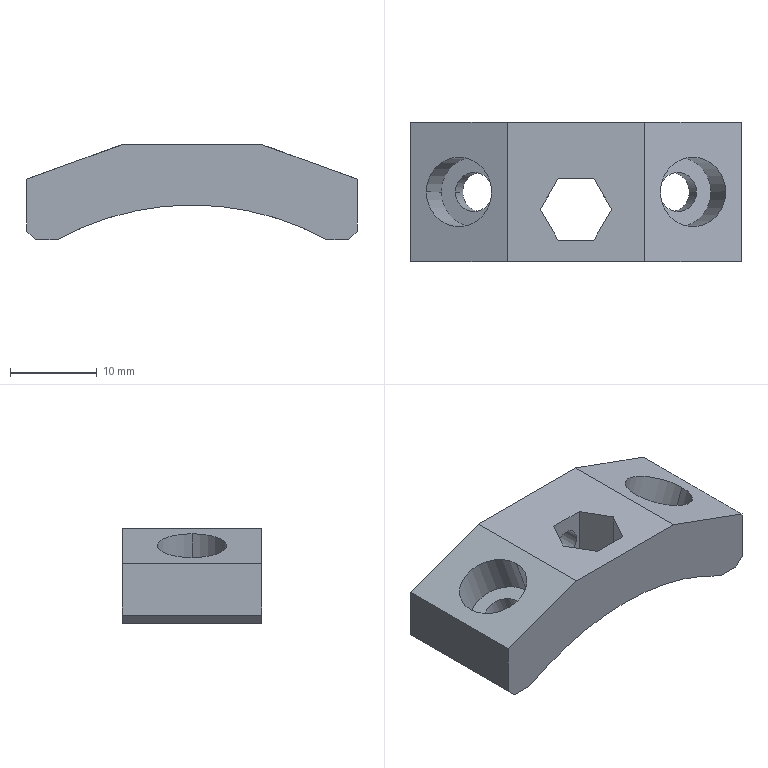Part | SolidWorks | features HoleWzd 2, Chamfer 1, Extrusion 1, ICE 1, MirrorPattern 1 | 1 solid | 30 faces | box 38 x 16 x 11 mm | volume 3676 mm3 | plane 19 | cylinder 11 | commonest cylinder face diameters 4.5 x4 8 x4 3.3 x2 64 x1
STEP:
#1=CARTESIAN_POINT('',(7.992,0.,33.654));
#2=VERTEX_POINT('',#1);
#3=CARTESIAN_POINT('',(15.51,0.,30.917));
#4=VERTEX_POINT('',#3);
#5=CARTESIAN_POINT('',(11.751,0.,32.286));
#6=DIRECTION('',(0.342,0.,0.9397));
#7=DIRECTION('',(0.9397,0.,-0.342));
#8=AXIS2_PLACEMENT_3D('',#5,#6,#7);
#9=CIRCLE('',#8,4.);
#10=EDGE_CURVE('',#2,#4,#9,.T.);
#11=ORIENTED_EDGE('',*,*,#10,.F.);
#12=CARTESIAN_POINT('',(9.702,0.,38.352));
#13=VERTEX_POINT('',#12);
#14=CARTESIAN_POINT('',(9.702,0.,38.352));
#15=DIRECTION('',(0.342,0.,0.9397));
#16=VECTOR('',#15,1000.);
#17=LINE('',#14,#16);
#18=EDGE_CURVE('',#2,#13,#17,.T.);
#19=ORIENTED_EDGE('',*,*,#18,.T.);
#20=CARTESIAN_POINT('',(17.22,0.,35.616));
#21=VERTEX_POINT('',#20);
#22=CARTESIAN_POINT('',(13.461,0.,36.984));
#23=DIRECTION('',(0.342,0.,0.9397));
#24=DIRECTION('',(0.9397,0.,-0.342));
#25=AXIS2_PLACEMENT_3D('',#22,#23,#24);
#26=CIRCLE('',#25,4.);
#27=EDGE_CURVE('',#13,#21,#26,.T.);
#28=ORIENTED_EDGE('',*,*,#27,.T.);
#29=CARTESIAN_POINT('',(17.22,0.,35.616));
#30=DIRECTION('',(0.342,0.,0.9397));
#31=VECTOR('',#30,1000.);
#32=LINE('',#29,#31);
#33=EDGE_CURVE('',#4,#21,#32,.T.);
#34=ORIENTED_EDGE('',*,*,#33,.F.);
#35=EDGE_LOOP('',(#11,#19,#28,#34));
#36=FACE_OUTER_BOUND('',#35,.T.);
#37=CARTESIAN_POINT('',(13.461,0.,36.984));
#38=DIRECTION('',(0.342,0.,0.9397));
#39=DIRECTION('',(0.9397,0.,-0.342));
#40=AXIS2_PLACEMENT_3D('',#37,#38,#39);
#41=CYLINDRICAL_SURFACE('',#40,4.);
#42=ADVANCED_FACE('',(#36),#41,.F.);
#43=CARTESIAN_POINT('',(8.803,0.,30.765));
#44=VERTEX_POINT('',#43);
#45=CARTESIAN_POINT('',(13.032,0.,29.226));
#46=VERTEX_POINT('',#45);
#47=CARTESIAN_POINT('',(8.803,0.,30.765));
#48=CARTESIAN_POINT('',(8.803,-0.1468,30.765));
#49=CARTESIAN_POINT('',(8.817,-0.2928,30.761));
#50=CARTESIAN_POINT('',(8.872,-0.583,30.745));
#51=CARTESIAN_POINT('',(8.914,-0.7251,30.733));
#52=CARTESIAN_POINT('',(9.076,-1.131,30.686));
#53=CARTESIAN_POINT('',(9.237,-1.382,30.639));
#54=CARTESIAN_POINT('',(9.534,-1.694,30.547));
#55=CARTESIAN_POINT('',(9.645,-1.789,30.512));
#56=CARTESIAN_POINT('',(9.878,-1.952,30.438));
#57=CARTESIAN_POINT('',(10.001,-2.021,30.398));
#58=CARTESIAN_POINT('',(10.259,-2.134,30.311));
#59=CARTESIAN_POINT('',(10.394,-2.178,30.265));
#60=CARTESIAN_POINT('',(10.666,-2.235,30.171));
#61=CARTESIAN_POINT('',(10.803,-2.25,30.122));
#62=CARTESIAN_POINT('',(11.082,-2.25,30.02));
#63=CARTESIAN_POINT('',(11.22,-2.236,29.969));
#64=CARTESIAN_POINT('',(11.489,-2.179,29.867));
#65=CARTESIAN_POINT('',(11.622,-2.136,29.815));
#66=CARTESIAN_POINT('',(11.876,-2.023,29.715));
#67=CARTESIAN_POINT('',(11.996,-1.954,29.667));
#68=CARTESIAN_POINT('',(12.222,-1.791,29.574));
#69=CARTESIAN_POINT('',(12.329,-1.696,29.53));
#70=CARTESIAN_POINT('',(12.521,-1.488,29.449));
#71=CARTESIAN_POINT('',(12.607,-1.375,29.412));
#72=CARTESIAN_POINT('',(12.758,-1.13,29.347));
#73=CARTESIAN_POINT('',(12.822,-0.9987,29.319));
#74=CARTESIAN_POINT('',(12.977,-0.5928,29.251));
#75=CARTESIAN_POINT('',(13.032,-0.2974,29.226));
#76=CARTESIAN_POINT('',(13.032,0.,29.226));
#77=B_SPLINE_CURVE_WITH_KNOTS('',3,(#47,#48,#49,#50,#51,#52,#53,#54,#55,#56,#57,#58,#59,#60,#61,#62,#63,#64,#65,#66,#67,#68,#69,#70,#71,#72,#73,#74,#75,#76),.UNSPECIFIED.,.F.,.F.,(4,2,2,2,2,2,2,2,2,2,2,2,2,2,4),(0.007037,0.007476,0.007916,0.008795,0.009235,0.009675,0.01011,0.01055,0.01099,0.01143,0.01187,0.01231,0.01275,0.01319,0.01407),.UNSPECIFIED.);
#78=EDGE_CURVE('',#44,#46,#77,.T.);
#79=ORIENTED_EDGE('',*,*,#78,.F.);
#80=CARTESIAN_POINT('',(9.637,0.,33.055));
#81=VERTEX_POINT('',#80);
#82=CARTESIAN_POINT('',(11.347,0.,37.754));
#83=DIRECTION('',(0.342,0.,0.9397));
#84=VECTOR('',#83,1000.);
#85=LINE('',#82,#84);
#86=EDGE_CURVE('',#44,#81,#85,.T.);
#87=ORIENTED_EDGE('',*,*,#86,.T.);
#88=CARTESIAN_POINT('',(13.865,0.,31.516));
#89=VERTEX_POINT('',#88);
#90=CARTESIAN_POINT('',(11.751,0.,32.286));
#91=DIRECTION('',(0.342,0.,0.9397));
#92=DIRECTION('',(0.9397,0.,-0.342));
#93=AXIS2_PLACEMENT_3D('',#90,#91,#92);
#94=CIRCLE('',#93,2.25);
#95=EDGE_CURVE('',#81,#89,#94,.T.);
#96=ORIENTED_EDGE('',*,*,#95,.T.);
#97=CARTESIAN_POINT('',(15.575,0.,36.214));
#98=DIRECTION('',(0.342,0.,0.9397));
#99=VECTOR('',#98,1000.);
#100=LINE('',#97,#99);
#101=EDGE_CURVE('',#46,#89,#100,.T.);
#102=ORIENTED_EDGE('',*,*,#101,.F.);
#103=EDGE_LOOP('',(#79,#87,#96,#102));
#104=FACE_OUTER_BOUND('',#103,.T.);
#105=CARTESIAN_POINT('',(13.461,0.,36.984));
#106=DIRECTION('',(0.342,0.,0.9397));
#107=DIRECTION('',(0.9397,0.,-0.342));
#108=AXIS2_PLACEMENT_3D('',#105,#106,#107);
#109=CYLINDRICAL_SURFACE('',#108,2.25);
#110=ADVANCED_FACE('',(#104),#109,.F.);
#111=CARTESIAN_POINT('',(-15.51,0.,30.917));
#112=VERTEX_POINT('',#111);
#113=CARTESIAN_POINT('',(-7.992,0.,33.654));
#114=VERTEX_POINT('',#113);
#115=CARTESIAN_POINT('',(-11.751,0.,32.286));
#116=DIRECTION('',(-0.342,0.,0.9397));
#117=DIRECTION('',(0.9397,0.,0.342));
#118=AXIS2_PLACEMENT_3D('',#115,#116,#117);
#119=CIRCLE('',#118,4.);
#120=EDGE_CURVE('',#112,#114,#119,.T.);
#121=ORIENTED_EDGE('',*,*,#120,.F.);
#122=CARTESIAN_POINT('',(-17.22,0.,35.616));
#123=VERTEX_POINT('',#122);
#124=CARTESIAN_POINT('',(-17.22,0.,35.616));
#125=DIRECTION('',(-0.342,0.,0.9397));
#126=VECTOR('',#125,1000.);
#127=LINE('',#124,#126);
#128=EDGE_CURVE('',#112,#123,#127,.T.);
#129=ORIENTED_EDGE('',*,*,#128,.T.);
#130=CARTESIAN_POINT('',(-9.702,0.,38.352));
#131=VERTEX_POINT('',#130);
#132=CARTESIAN_POINT('',(-13.461,0.,36.984));
#133=DIRECTION('',(-0.342,0.,0.9397));
#134=DIRECTION('',(0.9397,0.,0.342));
#135=AXIS2_PLACEMENT_3D('',#132,#133,#134);
#136=CIRCLE('',#135,4.);
#137=EDGE_CURVE('',#123,#131,#136,.T.);
#138=ORIENTED_EDGE('',*,*,#137,.T.);
#139=CARTESIAN_POINT('',(-9.702,0.,38.352));
#140=DIRECTION('',(-0.342,0.,0.9397));
#141=VECTOR('',#140,1000.);
#142=LINE('',#139,#141);
#143=EDGE_CURVE('',#114,#131,#142,.T.);
#144=ORIENTED_EDGE('',*,*,#143,.F.);
#145=EDGE_LOOP('',(#121,#129,#138,#144));
#146=FACE_OUTER_BOUND('',#145,.T.);
#147=CARTESIAN_POINT('',(-13.461,0.,36.984));
#148=DIRECTION('',(-0.342,0.,0.9397));
#149=DIRECTION('',(0.9397,0.,0.342));
#150=AXIS2_PLACEMENT_3D('',#147,#148,#149);
#151=CYLINDRICAL_SURFACE('',#150,4.);
#152=ADVANCED_FACE('',(#146),#151,.F.);
#153=CARTESIAN_POINT('',(-13.032,0.,29.226));
#154=VERTEX_POINT('',#153);
#155=CARTESIAN_POINT('',(-8.803,0.,30.765));
#156=VERTEX_POINT('',#155);
#157=CARTESIAN_POINT('',(-13.032,0.,29.226));
#158=CARTESIAN_POINT('',(-13.032,-0.1468,29.226));
#159=CARTESIAN_POINT('',(-13.019,-0.2928,29.232));
#160=CARTESIAN_POINT('',(-12.966,-0.583,29.255));
#161=CARTESIAN_POINT('',(-12.927,-0.7251,29.273));
#162=CARTESIAN_POINT('',(-12.772,-1.131,29.341));
#163=CARTESIAN_POINT('',(-12.618,-1.382,29.408));
#164=CARTESIAN_POINT('',(-12.332,-1.694,29.529));
#165=CARTESIAN_POINT('',(-12.225,-1.789,29.573));
#166=CARTESIAN_POINT('',(-11.998,-1.952,29.666));
#167=CARTESIAN_POINT('',(-11.878,-2.021,29.714));
#168=CARTESIAN_POINT('',(-11.625,-2.134,29.814));
#169=CARTESIAN_POINT('',(-11.492,-2.178,29.866));
#170=CARTESIAN_POINT('',(-11.223,-2.235,29.968));
#171=CARTESIAN_POINT('',(-11.086,-2.25,30.019));
#172=CARTESIAN_POINT('',(-10.807,-2.25,30.12));
#173=CARTESIAN_POINT('',(-10.669,-2.236,30.17));
#174=CARTESIAN_POINT('',(-10.397,-2.179,30.264));
#175=CARTESIAN_POINT('',(-10.262,-2.136,30.31));
#176=CARTESIAN_POINT('',(-10.003,-2.023,30.397));
#177=CARTESIAN_POINT('',(-9.88,-1.954,30.437));
#178=CARTESIAN_POINT('',(-9.647,-1.791,30.511));
#179=CARTESIAN_POINT('',(-9.537,-1.696,30.546));
#180=CARTESIAN_POINT('',(-9.338,-1.488,30.607));
#181=CARTESIAN_POINT('',(-9.248,-1.375,30.634));
#182=CARTESIAN_POINT('',(-9.091,-1.13,30.682));
#183=CARTESIAN_POINT('',(-9.023,-0.9987,30.702));
#184=CARTESIAN_POINT('',(-8.861,-0.5928,30.749));
#185=CARTESIAN_POINT('',(-8.803,-0.2974,30.765));
#186=CARTESIAN_POINT('',(-8.803,0.,30.765));
#187=B_SPLINE_CURVE_WITH_KNOTS('',3,(#157,#158,#159,#160,#161,#162,#163,#164,#165,#166,#167,#168,#169,#170,#171,#172,#173,#174,#175,#176,#177,#178,#179,#180,#181,#182,#183,#184,#185,#186),.UNSPECIFIED.,.F.,.F.,(4,2,2,2,2,2,2,2,2,2,2,2,2,2,4),(0.007037,0.007476,0.007916,0.008795,0.009235,0.009675,0.01011,0.01055,0.01099,0.01143,0.01187,0.01231,0.01275,0.01319,0.01407),.UNSPECIFIED.);
#188=EDGE_CURVE('',#154,#156,#187,.T.);
#189=ORIENTED_EDGE('',*,*,#188,.F.);
#190=CARTESIAN_POINT('',(-13.865,0.,31.516));
#191=VERTEX_POINT('',#190);
#192=CARTESIAN_POINT('',(-15.575,0.,36.214));
#193=DIRECTION('',(-0.342,0.,0.9397));
#194=VECTOR('',#193,1000.);
#195=LINE('',#192,#194);
#196=EDGE_CURVE('',#154,#191,#195,.T.);
#197=ORIENTED_EDGE('',*,*,#196,.T.);
#198=CARTESIAN_POINT('',(-9.637,0.,33.055));
#199=VERTEX_POINT('',#198);
#200=CARTESIAN_POINT('',(-11.751,0.,32.286));
#201=DIRECTION('',(-0.342,0.,0.9397));
#202=DIRECTION('',(0.9397,0.,0.342));
#203=AXIS2_PLACEMENT_3D('',#200,#201,#202);
#204=CIRCLE('',#203,2.25);
#205=EDGE_CURVE('',#191,#199,#204,.T.);
#206=ORIENTED_EDGE('',*,*,#205,.T.);
#207=CARTESIAN_POINT('',(-11.347,0.,37.754));
#208=DIRECTION('',(-0.342,0.,0.9397));
#209=VECTOR('',#208,1000.);
#210=LINE('',#207,#209);
#211=EDGE_CURVE('',#156,#199,#210,.T.);
#212=ORIENTED_EDGE('',*,*,#211,.F.);
#213=EDGE_LOOP('',(#189,#197,#206,#212));
#214=FACE_OUTER_BOUND('',#213,.T.);
#215=CARTESIAN_POINT('',(-13.461,0.,36.984));
#216=DIRECTION('',(-0.342,0.,0.9397));
#217=DIRECTION('',(0.9397,0.,0.342));
#218=AXIS2_PLACEMENT_3D('',#215,#216,#217);
#219=CYLINDRICAL_SURFACE('',#218,2.25);
#220=ADVANCED_FACE('',(#214),#219,.F.);
#221=CARTESIAN_POINT('',(0.,1.55,33.85));
#222=VERTEX_POINT('',#221);
#223=CARTESIAN_POINT('',(0.,1.55,37.15));
#224=VERTEX_POINT('',#223);
#225=CARTESIAN_POINT('',(0.,1.55,35.5));
#226=DIRECTION('',(0.,1.,0.));
#227=DIRECTION('',(-1.,0.,0.));
#228=AXIS2_PLACEMENT_3D('',#225,#226,#227);
#229=CIRCLE('',#228,1.65);
#230=EDGE_CURVE('',#222,#224,#229,.T.);
#231=ORIENTED_EDGE('',*,*,#230,.F.);
#232=CARTESIAN_POINT('',(0.,8.,33.85));
#233=VERTEX_POINT('',#232);
#234=CARTESIAN_POINT('',(0.,8.,33.85));
#235=DIRECTION('',(0.,1.,0.));
#236=VECTOR('',#235,1000.);
#237=LINE('',#234,#236);
#238=EDGE_CURVE('',#222,#233,#237,.T.);
#239=ORIENTED_EDGE('',*,*,#238,.T.);
#240=CARTESIAN_POINT('',(0.,8.,37.15));
#241=VERTEX_POINT('',#240);
#242=CARTESIAN_POINT('',(0.,8.,35.5));
#243=DIRECTION('',(0.,1.,0.));
#244=DIRECTION('',(0.,0.,1.));
#245=AXIS2_PLACEMENT_3D('',#242,#243,#244);
#246=CIRCLE('',#245,1.65);
#247=EDGE_CURVE('',#233,#241,#246,.T.);
#248=ORIENTED_EDGE('',*,*,#247,.T.);
#249=CARTESIAN_POINT('',(0.,8.,37.15));
#250=DIRECTION('',(0.,1.,0.));
#251=VECTOR('',#250,1000.);
#252=LINE('',#249,#251);
#253=EDGE_CURVE('',#224,#241,#252,.T.);
#254=ORIENTED_EDGE('',*,*,#253,.F.);
#255=EDGE_LOOP('',(#231,#239,#248,#254));
#256=FACE_OUTER_BOUND('',#255,.T.);
#257=CARTESIAN_POINT('',(0.,8.,35.5));
#258=DIRECTION('',(0.,1.,0.));
#259=DIRECTION('',(0.,0.,1.));
#260=AXIS2_PLACEMENT_3D('',#257,#258,#259);
#261=CYLINDRICAL_SURFACE('',#260,1.65);
#262=ADVANCED_FACE('',(#256),#261,.F.);
#263=CARTESIAN_POINT('',(-13.461,0.,36.984));
#264=DIRECTION('',(-0.342,0.,0.9397));
#265=DIRECTION('',(0.9397,0.,0.342));
#266=AXIS2_PLACEMENT_3D('',#263,#264,#265);
#267=CIRCLE('',#266,4.);
#268=EDGE_CURVE('',#131,#123,#267,.T.);
#269=ORIENTED_EDGE('',*,*,#268,.F.);
#270=ORIENTED_EDGE('',*,*,#137,.F.);
#271=EDGE_LOOP('',(#269,#270));
#272=FACE_BOUND('',#271,.T.);
#273=CARTESIAN_POINT('',(-19.,-8.,34.968));
#274=VERTEX_POINT('',#273);
#275=CARTESIAN_POINT('',(-7.922,-8.,39.));
#276=VERTEX_POINT('',#275);
#277=CARTESIAN_POINT('',(-7.922,-8.,39.));
#278=DIRECTION('',(0.9397,0.,0.342));
#279=VECTOR('',#278,1000.);
#280=LINE('',#277,#279);
#281=EDGE_CURVE('',#274,#276,#280,.T.);
#282=ORIENTED_EDGE('',*,*,#281,.T.);
#283=CARTESIAN_POINT('',(-7.922,8.,39.));
#284=VERTEX_POINT('',#283);
#285=CARTESIAN_POINT('',(-7.922,8.,39.));
#286=DIRECTION('',(0.,-1.,0.));
#287=VECTOR('',#286,1000.);
#288=LINE('',#285,#287);
#289=EDGE_CURVE('',#284,#276,#288,.T.);
#290=ORIENTED_EDGE('',*,*,#289,.F.);
#291=CARTESIAN_POINT('',(-19.,8.,34.968));
#292=VERTEX_POINT('',#291);
#293=CARTESIAN_POINT('',(-7.922,8.,39.));
#294=DIRECTION('',(0.9397,0.,0.342));
#295=VECTOR('',#294,1000.);
#296=LINE('',#293,#295);
#297=EDGE_CURVE('',#292,#284,#296,.T.);
#298=ORIENTED_EDGE('',*,*,#297,.F.);
#299=CARTESIAN_POINT('',(-19.,8.,34.968));
#300=DIRECTION('',(0.,-1.,0.));
#301=VECTOR('',#300,1000.);
#302=LINE('',#299,#301);
#303=EDGE_CURVE('',#292,#274,#302,.T.);
#304=ORIENTED_EDGE('',*,*,#303,.T.);
#305=EDGE_LOOP('',(#282,#290,#298,#304));
#306=FACE_OUTER_BOUND('',#305,.T.);
#307=CARTESIAN_POINT('',(-7.922,8.,39.));
#308=DIRECTION('',(0.342,0.,-0.9397));
#309=DIRECTION('',(-0.9397,0.,-0.342));
#310=AXIS2_PLACEMENT_3D('',#307,#308,#309);
#311=PLANE('',#310);
#312=ADVANCED_FACE('',(#272,#306),#311,.F.);
#313=CARTESIAN_POINT('',(4.099,-2.,39.));
#314=VERTEX_POINT('',#313);
#315=CARTESIAN_POINT('',(2.05,1.55,39.));
#316=VERTEX_POINT('',#315);
#317=CARTESIAN_POINT('',(4.099,-2.,39.));
#318=DIRECTION('',(-0.5,0.866,0.));
#319=VECTOR('',#318,1000.);
#320=LINE('',#317,#319);
#321=EDGE_CURVE('',#314,#316,#320,.T.);
#322=ORIENTED_EDGE('',*,*,#321,.F.);
#323=CARTESIAN_POINT('',(2.05,-5.55,39.));
#324=VERTEX_POINT('',#323);
#325=CARTESIAN_POINT('',(2.05,-5.55,39.));
#326=DIRECTION('',(0.5,0.866,0.));
#327=VECTOR('',#326,1000.);
#328=LINE('',#325,#327);
#329=EDGE_CURVE('',#324,#314,#328,.T.);
#330=ORIENTED_EDGE('',*,*,#329,.F.);
#331=CARTESIAN_POINT('',(-2.05,-5.55,39.));
#332=VERTEX_POINT('',#331);
#333=CARTESIAN_POINT('',(-2.05,-5.55,39.));
#334=DIRECTION('',(1.,0.,0.));
#335=VECTOR('',#334,1000.);
#336=LINE('',#333,#335);
#337=EDGE_CURVE('',#332,#324,#336,.T.);
#338=ORIENTED_EDGE('',*,*,#337,.F.);
#339=CARTESIAN_POINT('',(-4.099,-2.,39.));
#340=VERTEX_POINT('',#339);
#341=CARTESIAN_POINT('',(-4.099,-2.,39.));
#342=DIRECTION('',(0.5,-0.866,0.));
#343=VECTOR('',#342,1000.);
#344=LINE('',#341,#343);
#345=EDGE_CURVE('',#340,#332,#344,.T.);
#346=ORIENTED_EDGE('',*,*,#345,.F.);
#347=CARTESIAN_POINT('',(-2.05,1.55,39.));
#348=VERTEX_POINT('',#347);
#349=CARTESIAN_POINT('',(-2.05,1.55,39.));
#350=DIRECTION('',(-0.5,-0.866,0.));
#351=VECTOR('',#350,1000.);
#352=LINE('',#349,#351);
#353=EDGE_CURVE('',#348,#340,#352,.T.);
#354=ORIENTED_EDGE('',*,*,#353,.F.);
#355=CARTESIAN_POINT('',(2.05,1.55,39.));
#356=DIRECTION('',(-1.,0.,0.));
#357=VECTOR('',#356,1000.);
#358=LINE('',#355,#357);
#359=EDGE_CURVE('',#316,#348,#358,.T.);
#360=ORIENTED_EDGE('',*,*,#359,.F.);
#361=EDGE_LOOP('',(#322,#330,#338,#346,#354,#360));
#362=FACE_BOUND('',#361,.T.);
#363=CARTESIAN_POINT('',(7.922,-8.,39.));
#364=VERTEX_POINT('',#363);
#365=CARTESIAN_POINT('',(-7.922,-8.,39.));
#366=DIRECTION('',(1.,0.,0.));
#367=VECTOR('',#366,1000.);
#368=LINE('',#365,#367);
#369=EDGE_CURVE('',#276,#364,#368,.T.);
#370=ORIENTED_EDGE('',*,*,#369,.T.);
#371=CARTESIAN_POINT('',(7.922,8.,39.));
#372=VERTEX_POINT('',#371);
#373=CARTESIAN_POINT('',(7.922,8.,39.));
#374=DIRECTION('',(0.,-1.,0.));
#375=VECTOR('',#374,1000.);
#376=LINE('',#373,#375);
#377=EDGE_CURVE('',#372,#364,#376,.T.);
#378=ORIENTED_EDGE('',*,*,#377,.F.);
#379=CARTESIAN_POINT('',(-7.922,8.,39.));
#380=DIRECTION('',(1.,0.,0.));
#381=VECTOR('',#380,1000.);
#382=LINE('',#379,#381);
#383=EDGE_CURVE('',#284,#372,#382,.T.);
#384=ORIENTED_EDGE('',*,*,#383,.F.);
#385=ORIENTED_EDGE('',*,*,#289,.T.);
#386=EDGE_LOOP('',(#370,#378,#384,#385));
#387=FACE_OUTER_BOUND('',#386,.T.);
#388=CARTESIAN_POINT('',(-7.922,8.,39.));
#389=DIRECTION('',(0.,0.,-1.));
#390=DIRECTION('',(-1.,0.,0.));
#391=AXIS2_PLACEMENT_3D('',#388,#389,#390);
#392=PLANE('',#391);
#393=ADVANCED_FACE('',(#362,#387),#392,.F.);
#394=CARTESIAN_POINT('',(13.461,0.,36.984));
#395=DIRECTION('',(0.342,0.,0.9397));
#396=DIRECTION('',(0.9397,0.,-0.342));
#397=AXIS2_PLACEMENT_3D('',#394,#395,#396);
#398=CIRCLE('',#397,4.);
#399=EDGE_CURVE('',#21,#13,#398,.T.);
#400=ORIENTED_EDGE('',*,*,#399,.F.);
#401=ORIENTED_EDGE('',*,*,#27,.F.);
#402=EDGE_LOOP('',(#400,#401));
#403=FACE_BOUND('',#402,.T.);
#404=CARTESIAN_POINT('',(19.,-8.,34.968));
#405=VERTEX_POINT('',#404);
#406=CARTESIAN_POINT('',(7.922,-8.,39.));
#407=DIRECTION('',(0.9397,0.,-0.342));
#408=VECTOR('',#407,1000.);
#409=LINE('',#406,#408);
#410=EDGE_CURVE('',#364,#405,#409,.T.);
#411=ORIENTED_EDGE('',*,*,#410,.T.);
#412=CARTESIAN_POINT('',(19.,8.,34.968));
#413=VERTEX_POINT('',#412);
#414=CARTESIAN_POINT('',(19.,8.,34.968));
#415=DIRECTION('',(0.,-1.,0.));
#416=VECTOR('',#415,1000.);
#417=LINE('',#414,#416);
#418=EDGE_CURVE('',#413,#405,#417,.T.);
#419=ORIENTED_EDGE('',*,*,#418,.F.);
#420=CARTESIAN_POINT('',(7.922,8.,39.));
#421=DIRECTION('',(0.9397,0.,-0.342));
#422=VECTOR('',#421,1000.);
#423=LINE('',#420,#422);
#424=EDGE_CURVE('',#372,#413,#423,.T.);
#425=ORIENTED_EDGE('',*,*,#424,.F.);
#426=ORIENTED_EDGE('',*,*,#377,.T.);
#427=EDGE_LOOP('',(#411,#419,#425,#426));
#428=FACE_OUTER_BOUND('',#427,.T.);
#429=CARTESIAN_POINT('',(7.922,8.,39.));
#430=DIRECTION('',(-0.342,0.,-0.9397));
#431=DIRECTION('',(-0.9397,0.,0.342));
#432=AXIS2_PLACEMENT_3D('',#429,#430,#431);
#433=PLANE('',#432);
#434=ADVANCED_FACE('',(#403,#428),#433,.F.);
#435=CARTESIAN_POINT('',(19.,-8.,29.));
#436=VERTEX_POINT('',#435);
#437=CARTESIAN_POINT('',(19.,-8.,28.));
#438=DIRECTION('',(0.,0.,-1.));
#439=VECTOR('',#438,1000.);
#440=LINE('',#437,#439);
#441=EDGE_CURVE('',#405,#436,#440,.T.);
#442=ORIENTED_EDGE('',*,*,#441,.T.);
#443=CARTESIAN_POINT('',(19.,8.,29.));
#444=VERTEX_POINT('',#443);
#445=CARTESIAN_POINT('',(19.,8.,29.));
#446=DIRECTION('',(0.,1.,0.));
#447=VECTOR('',#446,1000.);
#448=LINE('',#445,#447);
#449=EDGE_CURVE('',#436,#444,#448,.T.);
#450=ORIENTED_EDGE('',*,*,#449,.T.);
#451=CARTESIAN_POINT('',(19.,8.,28.));
#452=DIRECTION('',(0.,0.,-1.));
#453=VECTOR('',#452,1000.);
#454=LINE('',#451,#453);
#455=EDGE_CURVE('',#413,#444,#454,.T.);
#456=ORIENTED_EDGE('',*,*,#455,.F.);
#457=ORIENTED_EDGE('',*,*,#418,.T.);
#458=EDGE_LOOP('',(#442,#450,#456,#457));
#459=FACE_OUTER_BOUND('',#458,.T.);
#460=CARTESIAN_POINT('',(19.,8.,28.));
#461=DIRECTION('',(-1.,0.,0.));
#462=DIRECTION('',(0.,0.,1.));
#463=AXIS2_PLACEMENT_3D('',#460,#461,#462);
#464=PLANE('',#463);
#465=ADVANCED_FACE('',(#459),#464,.F.);
#466=CARTESIAN_POINT('',(18.,8.,28.));
#467=VERTEX_POINT('',#466);
#468=CARTESIAN_POINT('',(15.492,8.,28.));
#469=VERTEX_POINT('',#468);
#470=CARTESIAN_POINT('',(19.,8.,28.));
#471=DIRECTION('',(-1.,0.,0.));
#472=VECTOR('',#471,1000.);
#473=LINE('',#470,#472);
#474=EDGE_CURVE('',#467,#469,#473,.T.);
#475=ORIENTED_EDGE('',*,*,#474,.F.);
#476=CARTESIAN_POINT('',(18.,-8.,28.));
#477=VERTEX_POINT('',#476);
#478=CARTESIAN_POINT('',(18.,8.,28.));
#479=DIRECTION('',(0.,-1.,0.));
#480=VECTOR('',#479,1000.);
#481=LINE('',#478,#480);
#482=EDGE_CURVE('',#467,#477,#481,.T.);
#483=ORIENTED_EDGE('',*,*,#482,.T.);
#484=CARTESIAN_POINT('',(15.492,-8.,28.));
#485=VERTEX_POINT('',#484);
#486=CARTESIAN_POINT('',(19.,-8.,28.));
#487=DIRECTION('',(-1.,0.,0.));
#488=VECTOR('',#487,1000.);
#489=LINE('',#486,#488);
#490=EDGE_CURVE('',#477,#485,#489,.T.);
#491=ORIENTED_EDGE('',*,*,#490,.T.);
#492=CARTESIAN_POINT('',(15.492,8.,28.));
#493=DIRECTION('',(0.,-1.,0.));
#494=VECTOR('',#493,1000.);
#495=LINE('',#492,#494);
#496=EDGE_CURVE('',#469,#485,#495,.T.);
#497=ORIENTED_EDGE('',*,*,#496,.F.);
#498=EDGE_LOOP('',(#475,#483,#491,#497));
#499=FACE_OUTER_BOUND('',#498,.T.);
#500=CARTESIAN_POINT('',(19.,8.,28.));
#501=DIRECTION('',(0.,0.,1.));
#502=DIRECTION('',(1.,0.,0.));
#503=AXIS2_PLACEMENT_3D('',#500,#501,#502);
#504=PLANE('',#503);
#505=ADVANCED_FACE('',(#499),#504,.F.);
#506=CARTESIAN_POINT('',(13.032,0.,29.226));
#507=CARTESIAN_POINT('',(13.032,0.1487,29.226));
#508=CARTESIAN_POINT('',(13.019,0.2949,29.232));
#509=CARTESIAN_POINT('',(12.966,0.5826,29.255));
#510=CARTESIAN_POINT('',(12.926,0.7255,29.273));
#511=CARTESIAN_POINT('',(12.823,0.998,29.319));
#512=CARTESIAN_POINT('',(12.759,1.127,29.346));
#513=CARTESIAN_POINT('',(12.609,1.372,29.411));
#514=CARTESIAN_POINT('',(12.522,1.488,29.449));
#515=CARTESIAN_POINT('',(12.234,1.799,29.57));
#516=CARTESIAN_POINT('',(12.002,1.966,29.665));
#517=CARTESIAN_POINT('',(11.498,2.191,29.864));
#518=CARTESIAN_POINT('',(11.221,2.25,29.969));
#519=CARTESIAN_POINT('',(10.807,2.25,30.12));
#520=CARTESIAN_POINT('',(10.667,2.235,30.17));
#521=CARTESIAN_POINT('',(10.394,2.178,30.265));
#522=CARTESIAN_POINT('',(10.262,2.135,30.31));
#523=CARTESIAN_POINT('',(10.003,2.023,30.397));
#524=CARTESIAN_POINT('',(9.878,1.952,30.438));
#525=CARTESIAN_POINT('',(9.645,1.789,30.512));
#526=CARTESIAN_POINT('',(9.537,1.696,30.546));
#527=CARTESIAN_POINT('',(9.336,1.486,30.608));
#528=CARTESIAN_POINT('',(9.247,1.373,30.635));
#529=CARTESIAN_POINT('',(9.09,1.129,30.682));
#530=CARTESIAN_POINT('',(9.022,0.9973,30.702));
#531=CARTESIAN_POINT('',(8.914,0.7247,30.733));
#532=CARTESIAN_POINT('',(8.873,0.5844,30.745));
#533=CARTESIAN_POINT('',(8.817,0.296,30.761));
#534=CARTESIAN_POINT('',(8.803,0.1469,30.765));
#535=CARTESIAN_POINT('',(8.803,0.,30.765));
#536=B_SPLINE_CURVE_WITH_KNOTS('',3,(#506,#507,#508,#509,#510,#511,#512,#513,#514,#515,#516,#517,#518,#519,#520,#521,#522,#523,#524,#525,#526,#527,#528,#529,#530,#531,#532,#533,#534,#535),.UNSPECIFIED.,.F.,.F.,(4,2,2,2,2,2,2,2,2,2,2,2,2,2,4),(0.,0.0004398,0.0008796,0.001319,0.001759,0.002639,0.003518,0.003958,0.004398,0.004838,0.005278,0.005717,0.006157,0.006597,0.007037),.UNSPECIFIED.);
#537=EDGE_CURVE('',#46,#44,#536,.T.);
#538=ORIENTED_EDGE('',*,*,#537,.T.);
#539=ORIENTED_EDGE('',*,*,#78,.T.);
#540=EDGE_LOOP('',(#538,#539));
#541=FACE_BOUND('',#540,.T.);
#542=CARTESIAN_POINT('',(-8.803,0.,30.765));
#543=CARTESIAN_POINT('',(-8.803,0.1487,30.765));
#544=CARTESIAN_POINT('',(-8.817,0.2949,30.761));
#545=CARTESIAN_POINT('',(-8.872,0.5826,30.745));
#546=CARTESIAN_POINT('',(-8.914,0.7255,30.733));
#547=CARTESIAN_POINT('',(-9.023,0.998,30.702));
#548=CARTESIAN_POINT('',(-9.089,1.127,30.682));
#549=CARTESIAN_POINT('',(-9.246,1.372,30.635));
#550=CARTESIAN_POINT('',(-9.337,1.488,30.608));
#551=CARTESIAN_POINT('',(-9.635,1.799,30.516));
#552=CARTESIAN_POINT('',(-9.874,1.966,30.44));
#553=CARTESIAN_POINT('',(-10.388,2.191,30.268));
#554=CARTESIAN_POINT('',(-10.668,2.25,30.171));
#555=CARTESIAN_POINT('',(-11.082,2.25,30.02));
#556=CARTESIAN_POINT('',(-11.222,2.235,29.968));
#557=CARTESIAN_POINT('',(-11.491,2.178,29.866));
#558=CARTESIAN_POINT('',(-11.622,2.135,29.815));
#559=CARTESIAN_POINT('',(-11.876,2.023,29.715));
#560=CARTESIAN_POINT('',(-11.998,1.952,29.666));
#561=CARTESIAN_POINT('',(-12.224,1.789,29.573));
#562=CARTESIAN_POINT('',(-12.329,1.696,29.53));
#563=CARTESIAN_POINT('',(-12.523,1.486,29.448));
#564=CARTESIAN_POINT('',(-12.609,1.373,29.411));
#565=CARTESIAN_POINT('',(-12.758,1.129,29.347));
#566=CARTESIAN_POINT('',(-12.823,0.9973,29.318));
#567=CARTESIAN_POINT('',(-12.927,0.7247,29.273));
#568=CARTESIAN_POINT('',(-12.966,0.5844,29.256));
#569=CARTESIAN_POINT('',(-13.018,0.296,29.232));
#570=CARTESIAN_POINT('',(-13.032,0.1469,29.226));
#571=CARTESIAN_POINT('',(-13.032,0.,29.226));
#572=B_SPLINE_CURVE_WITH_KNOTS('',3,(#542,#543,#544,#545,#546,#547,#548,#549,#550,#551,#552,#553,#554,#555,#556,#557,#558,#559,#560,#561,#562,#563,#564,#565,#566,#567,#568,#569,#570,#571),.UNSPECIFIED.,.F.,.F.,(4,2,2,2,2,2,2,2,2,2,2,2,2,2,4),(0.,0.0004398,0.0008796,0.001319,0.001759,0.002639,0.003518,0.003958,0.004398,0.004838,0.005278,0.005717,0.006157,0.006597,0.007037),.UNSPECIFIED.);
#573=EDGE_CURVE('',#156,#154,#572,.T.);
#574=ORIENTED_EDGE('',*,*,#573,.T.);
#575=ORIENTED_EDGE('',*,*,#188,.T.);
#576=EDGE_LOOP('',(#574,#575));
#577=FACE_BOUND('',#576,.T.);
#578=CARTESIAN_POINT('',(-2.05,-5.55,31.934));
#579=VERTEX_POINT('',#578);
#580=CARTESIAN_POINT('',(2.05,-5.55,31.934));
#581=VERTEX_POINT('',#580);
#582=CARTESIAN_POINT('',(0.,-5.55,0.));
#583=DIRECTION('',(0.,1.,0.));
#584=DIRECTION('',(1.,0.,0.));
#585=AXIS2_PLACEMENT_3D('',#582,#583,#584);
#586=CIRCLE('',#585,32.);
#587=EDGE_CURVE('',#579,#581,#586,.T.);
#588=ORIENTED_EDGE('',*,*,#587,.T.);
#589=CARTESIAN_POINT('',(4.099,-2.,31.736));
#590=VERTEX_POINT('',#589);
#591=CARTESIAN_POINT('',(2.05,-5.55,31.934));
#592=CARTESIAN_POINT('',(2.735,-4.363,31.89));
#593=CARTESIAN_POINT('',(3.418,-3.179,31.824));
#594=CARTESIAN_POINT('',(4.099,-2.,31.736));
#595=(BOUNDED_CURVE()B_SPLINE_CURVE(3,(#591,#592,#593,#594),.UNSPECIFIED.,.F.,.F.)B_SPLINE_CURVE_WITH_KNOTS((4,4),(1.635,1.699),.UNSPECIFIED.)CURVE()GEOMETRIC_REPRESENTATION_ITEM()RATIONAL_B_SPLINE_CURVE((1.,0.9997,0.9997,1.))REPRESENTATION_ITEM(''));
#596=EDGE_CURVE('',#581,#590,#595,.T.);
#597=ORIENTED_EDGE('',*,*,#596,.T.);
#598=CARTESIAN_POINT('',(2.05,1.55,31.934));
#599=VERTEX_POINT('',#598);
#600=CARTESIAN_POINT('',(4.099,-2.,31.736));
#601=CARTESIAN_POINT('',(3.418,-0.8205,31.824));
#602=CARTESIAN_POINT('',(2.735,0.3632,31.89));
#603=CARTESIAN_POINT('',(2.05,1.55,31.934));
#604=(BOUNDED_CURVE()B_SPLINE_CURVE(3,(#600,#601,#602,#603),.UNSPECIFIED.,.F.,.F.)B_SPLINE_CURVE_WITH_KNOTS((4,4),(1.442,1.507),.UNSPECIFIED.)CURVE()GEOMETRIC_REPRESENTATION_ITEM()RATIONAL_B_SPLINE_CURVE((1.,0.9997,0.9997,1.))REPRESENTATION_ITEM(''));
#605=EDGE_CURVE('',#590,#599,#604,.T.);
#606=ORIENTED_EDGE('',*,*,#605,.T.);
#607=CARTESIAN_POINT('',(-2.05,1.55,31.934));
#608=VERTEX_POINT('',#607);
#609=CARTESIAN_POINT('',(0.,1.55,0.));
#610=DIRECTION('',(0.,-1.,0.));
#611=DIRECTION('',(-1.,0.,0.));
#612=AXIS2_PLACEMENT_3D('',#609,#610,#611);
#613=CIRCLE('',#612,32.);
#614=EDGE_CURVE('',#599,#608,#613,.T.);
#615=ORIENTED_EDGE('',*,*,#614,.T.);
#616=CARTESIAN_POINT('',(-4.099,-2.,31.736));
#617=VERTEX_POINT('',#616);
#618=CARTESIAN_POINT('',(-2.05,1.55,31.934));
#619=CARTESIAN_POINT('',(-2.735,0.3632,31.89));
#620=CARTESIAN_POINT('',(-3.418,-0.8205,31.824));
#621=CARTESIAN_POINT('',(-4.099,-2.,31.736));
#622=(BOUNDED_CURVE()B_SPLINE_CURVE(3,(#618,#619,#620,#621),.UNSPECIFIED.,.F.,.F.)B_SPLINE_CURVE_WITH_KNOTS((4,4),(4.776,4.841),.UNSPECIFIED.)CURVE()GEOMETRIC_REPRESENTATION_ITEM()RATIONAL_B_SPLINE_CURVE((1.,0.9997,0.9997,1.))REPRESENTATION_ITEM(''));
#623=EDGE_CURVE('',#608,#617,#622,.T.);
#624=ORIENTED_EDGE('',*,*,#623,.T.);
#625=CARTESIAN_POINT('',(-4.099,-2.,31.736));
#626=CARTESIAN_POINT('',(-3.418,-3.179,31.824));
#627=CARTESIAN_POINT('',(-2.735,-4.363,31.89));
#628=CARTESIAN_POINT('',(-2.05,-5.55,31.934));
#629=(BOUNDED_CURVE()B_SPLINE_CURVE(3,(#625,#626,#627,#628),.UNSPECIFIED.,.F.,.T.)B_SPLINE_CURVE_WITH_KNOTS((4,4),(4.584,4.648),.UNSPECIFIED.)CURVE()GEOMETRIC_REPRESENTATION_ITEM()RATIONAL_B_SPLINE_CURVE((1.,0.9997,0.9997,1.))REPRESENTATION_ITEM(''));
#630=EDGE_CURVE('',#617,#579,#629,.T.);
#631=ORIENTED_EDGE('',*,*,#630,.T.);
#632=EDGE_LOOP('',(#588,#597,#606,#615,#624,#631));
#633=FACE_BOUND('',#632,.T.);
#634=CARTESIAN_POINT('',(-15.492,-8.,28.));
#635=VERTEX_POINT('',#634);
#636=CARTESIAN_POINT('',(0.,-8.,0.));
#637=DIRECTION('',(0.,-1.,0.));
#638=DIRECTION('',(0.,0.,1.));
#639=AXIS2_PLACEMENT_3D('',#636,#637,#638);
#640=CIRCLE('',#639,32.);
#641=EDGE_CURVE('',#485,#635,#640,.T.);
#642=ORIENTED_EDGE('',*,*,#641,.T.);
#643=CARTESIAN_POINT('',(-15.492,8.,28.));
#644=VERTEX_POINT('',#643);
#645=CARTESIAN_POINT('',(-15.492,8.,28.));
#646=DIRECTION('',(0.,-1.,0.));
#647=VECTOR('',#646,1000.);
#648=LINE('',#645,#647);
#649=EDGE_CURVE('',#644,#635,#648,.T.);
#650=ORIENTED_EDGE('',*,*,#649,.F.);
#651=CARTESIAN_POINT('',(0.,8.,0.));
#652=DIRECTION('',(0.,-1.,0.));
#653=DIRECTION('',(0.,0.,1.));
#654=AXIS2_PLACEMENT_3D('',#651,#652,#653);
#655=CIRCLE('',#654,32.);
#656=EDGE_CURVE('',#469,#644,#655,.T.);
#657=ORIENTED_EDGE('',*,*,#656,.F.);
#658=ORIENTED_EDGE('',*,*,#496,.T.);
#659=EDGE_LOOP('',(#642,#650,#657,#658));
#660=FACE_OUTER_BOUND('',#659,.T.);
#661=CARTESIAN_POINT('',(0.,8.,0.));
#662=DIRECTION('',(0.,-1.,0.));
#663=DIRECTION('',(0.,0.,-1.));
#664=AXIS2_PLACEMENT_3D('',#661,#662,#663);
#665=CYLINDRICAL_SURFACE('',#664,32.);
#666=ADVANCED_FACE('',(#541,#577,#633,#660),#665,.F.);
#667=CARTESIAN_POINT('',(-18.,-8.,28.));
#668=VERTEX_POINT('',#667);
#669=CARTESIAN_POINT('',(-19.,-8.,28.));
#670=DIRECTION('',(-1.,0.,0.));
#671=VECTOR('',#670,1000.);
#672=LINE('',#669,#671);
#673=EDGE_CURVE('',#635,#668,#672,.T.);
#674=ORIENTED_EDGE('',*,*,#673,.T.);
#675=CARTESIAN_POINT('',(-18.,8.,28.));
#676=VERTEX_POINT('',#675);
#677=CARTESIAN_POINT('',(-18.,8.,28.));
#678=DIRECTION('',(0.,1.,0.));
#679=VECTOR('',#678,1000.);
#680=LINE('',#677,#679);
#681=EDGE_CURVE('',#668,#676,#680,.T.);
#682=ORIENTED_EDGE('',*,*,#681,.T.);
#683=CARTESIAN_POINT('',(-19.,8.,28.));
#684=DIRECTION('',(-1.,0.,0.));
#685=VECTOR('',#684,1000.);
#686=LINE('',#683,#685);
#687=EDGE_CURVE('',#644,#676,#686,.T.);
#688=ORIENTED_EDGE('',*,*,#687,.F.);
#689=ORIENTED_EDGE('',*,*,#649,.T.);
#690=EDGE_LOOP('',(#674,#682,#688,#689));
#691=FACE_OUTER_BOUND('',#690,.T.);
#692=CARTESIAN_POINT('',(-19.,8.,28.));
#693=DIRECTION('',(0.,0.,1.));
#694=DIRECTION('',(1.,0.,0.));
#695=AXIS2_PLACEMENT_3D('',#692,#693,#694);
#696=PLANE('',#695);
#697=ADVANCED_FACE('',(#691),#696,.F.);
#698=CARTESIAN_POINT('',(-19.,8.,29.));
#699=VERTEX_POINT('',#698);
#700=CARTESIAN_POINT('',(-19.,8.,28.));
#701=DIRECTION('',(0.,0.,1.));
#702=VECTOR('',#701,1000.);
#703=LINE('',#700,#702);
#704=EDGE_CURVE('',#699,#292,#703,.T.);
#705=ORIENTED_EDGE('',*,*,#704,.F.);
#706=CARTESIAN_POINT('',(-19.,-8.,29.));
#707=VERTEX_POINT('',#706);
#708=CARTESIAN_POINT('',(-19.,8.,29.));
#709=DIRECTION('',(0.,-1.,0.));
#710=VECTOR('',#709,1000.);
#711=LINE('',#708,#710);
#712=EDGE_CURVE('',#699,#707,#711,.T.);
#713=ORIENTED_EDGE('',*,*,#712,.T.);
#714=CARTESIAN_POINT('',(-19.,-8.,28.));
#715=DIRECTION('',(0.,0.,1.));
#716=VECTOR('',#715,1000.);
#717=LINE('',#714,#716);
#718=EDGE_CURVE('',#707,#274,#717,.T.);
#719=ORIENTED_EDGE('',*,*,#718,.T.);
#720=ORIENTED_EDGE('',*,*,#303,.F.);
#721=EDGE_LOOP('',(#705,#713,#719,#720));
#722=FACE_OUTER_BOUND('',#721,.T.);
#723=CARTESIAN_POINT('',(-19.,8.,28.));
#724=DIRECTION('',(1.,0.,0.));
#725=DIRECTION('',(0.,0.,-1.));
#726=AXIS2_PLACEMENT_3D('',#723,#724,#725);
#727=PLANE('',#726);
#728=ADVANCED_FACE('',(#722),#727,.F.);
#729=CARTESIAN_POINT('',(0.,8.,35.5));
#730=DIRECTION('',(0.,1.,0.));
#731=DIRECTION('',(0.,0.,1.));
#732=AXIS2_PLACEMENT_3D('',#729,#730,#731);
#733=CIRCLE('',#732,1.65);
#734=EDGE_CURVE('',#241,#233,#733,.T.);
#735=ORIENTED_EDGE('',*,*,#734,.F.);
#736=ORIENTED_EDGE('',*,*,#247,.F.);
#737=EDGE_LOOP('',(#735,#736));
#738=FACE_BOUND('',#737,.T.);
#739=ORIENTED_EDGE('',*,*,#455,.T.);
#740=CARTESIAN_POINT('',(-5.,8.,5.));
#741=DIRECTION('',(-0.7071,0.,-0.7071));
#742=VECTOR('',#741,1000.);
#743=LINE('',#740,#742);
#744=EDGE_CURVE('',#444,#467,#743,.T.);
#745=ORIENTED_EDGE('',*,*,#744,.T.);
#746=ORIENTED_EDGE('',*,*,#474,.T.);
#747=ORIENTED_EDGE('',*,*,#656,.T.);
#748=ORIENTED_EDGE('',*,*,#687,.T.);
#749=CARTESIAN_POINT('',(5.,8.,5.));
#750=DIRECTION('',(-0.7071,0.,0.7071));
#751=VECTOR('',#750,1000.);
#752=LINE('',#749,#751);
#753=EDGE_CURVE('',#676,#699,#752,.T.);
#754=ORIENTED_EDGE('',*,*,#753,.T.);
#755=ORIENTED_EDGE('',*,*,#704,.T.);
#756=ORIENTED_EDGE('',*,*,#297,.T.);
#757=ORIENTED_EDGE('',*,*,#383,.T.);
#758=ORIENTED_EDGE('',*,*,#424,.T.);
#759=EDGE_LOOP('',(#739,#745,#746,#747,#748,#754,#755,#756,#757,#758));
#760=FACE_OUTER_BOUND('',#759,.T.);
#761=CARTESIAN_POINT('',(0.,8.,0.));
#762=DIRECTION('',(0.,1.,0.));
#763=DIRECTION('',(0.,0.,1.));
#764=AXIS2_PLACEMENT_3D('',#761,#762,#763);
#765=PLANE('',#764);
#766=ADVANCED_FACE('',(#738,#760),#765,.T.);
#767=ORIENTED_EDGE('',*,*,#490,.F.);
#768=CARTESIAN_POINT('',(18.,-8.,28.));
#769=DIRECTION('',(0.7071,0.,0.7071));
#770=VECTOR('',#769,1000.);
#771=LINE('',#768,#770);
#772=EDGE_CURVE('',#477,#436,#771,.T.);
#773=ORIENTED_EDGE('',*,*,#772,.T.);
#774=ORIENTED_EDGE('',*,*,#441,.F.);
#775=ORIENTED_EDGE('',*,*,#410,.F.);
#776=ORIENTED_EDGE('',*,*,#369,.F.);
#777=ORIENTED_EDGE('',*,*,#281,.F.);
#778=ORIENTED_EDGE('',*,*,#718,.F.);
#779=CARTESIAN_POINT('',(-19.,-8.,29.));
#780=DIRECTION('',(0.7071,0.,-0.7071));
#781=VECTOR('',#780,1000.);
#782=LINE('',#779,#781);
#783=EDGE_CURVE('',#707,#668,#782,.T.);
#784=ORIENTED_EDGE('',*,*,#783,.T.);
#785=ORIENTED_EDGE('',*,*,#673,.F.);
#786=ORIENTED_EDGE('',*,*,#641,.F.);
#787=EDGE_LOOP('',(#767,#773,#774,#775,#776,#777,#778,#784,#785,#786));
#788=FACE_OUTER_BOUND('',#787,.T.);
#789=CARTESIAN_POINT('',(0.,-8.,0.));
#790=DIRECTION('',(0.,1.,0.));
#791=DIRECTION('',(0.,0.,1.));
#792=AXIS2_PLACEMENT_3D('',#789,#790,#791);
#793=PLANE('',#792);
#794=ADVANCED_FACE('',(#788),#793,.F.);
#795=CARTESIAN_POINT('',(2.05,-5.55,28.));
#796=DIRECTION('',(0.,0.,1.));
#797=VECTOR('',#796,1000.);
#798=LINE('',#795,#797);
#799=EDGE_CURVE('',#581,#324,#798,.T.);
#800=ORIENTED_EDGE('',*,*,#799,.T.);
#801=ORIENTED_EDGE('',*,*,#329,.T.);
#802=CARTESIAN_POINT('',(4.099,-2.,28.));
#803=DIRECTION('',(0.,0.,1.));
#804=VECTOR('',#803,1000.);
#805=LINE('',#802,#804);
#806=EDGE_CURVE('',#590,#314,#805,.T.);
#807=ORIENTED_EDGE('',*,*,#806,.F.);
#808=ORIENTED_EDGE('',*,*,#596,.F.);
#809=EDGE_LOOP('',(#800,#801,#807,#808));
#810=FACE_OUTER_BOUND('',#809,.T.);
#811=CARTESIAN_POINT('',(2.05,-5.55,28.));
#812=DIRECTION('',(0.866,-0.5,0.));
#813=DIRECTION('',(0.5,0.866,0.));
#814=AXIS2_PLACEMENT_3D('',#811,#812,#813);
#815=PLANE('',#814);
#816=ADVANCED_FACE('',(#810),#815,.F.);
#817=CARTESIAN_POINT('',(-2.05,-5.55,28.));
#818=DIRECTION('',(0.,0.,1.));
#819=VECTOR('',#818,1000.);
#820=LINE('',#817,#819);
#821=EDGE_CURVE('',#579,#332,#820,.T.);
#822=ORIENTED_EDGE('',*,*,#821,.T.);
#823=ORIENTED_EDGE('',*,*,#337,.T.);
#824=ORIENTED_EDGE('',*,*,#799,.F.);
#825=ORIENTED_EDGE('',*,*,#587,.F.);
#826=EDGE_LOOP('',(#822,#823,#824,#825));
#827=FACE_OUTER_BOUND('',#826,.T.);
#828=CARTESIAN_POINT('',(-2.05,-5.55,28.));
#829=DIRECTION('',(0.,-1.,0.));
#830=DIRECTION('',(1.,0.,0.));
#831=AXIS2_PLACEMENT_3D('',#828,#829,#830);
#832=PLANE('',#831);
#833=ADVANCED_FACE('',(#827),#832,.F.);
#834=CARTESIAN_POINT('',(-4.099,-2.,28.));
#835=DIRECTION('',(0.,0.,1.));
#836=VECTOR('',#835,1000.);
#837=LINE('',#834,#836);
#838=EDGE_CURVE('',#617,#340,#837,.T.);
#839=ORIENTED_EDGE('',*,*,#838,.T.);
#840=ORIENTED_EDGE('',*,*,#345,.T.);
#841=ORIENTED_EDGE('',*,*,#821,.F.);
#842=ORIENTED_EDGE('',*,*,#630,.F.);
#843=EDGE_LOOP('',(#839,#840,#841,#842));
#844=FACE_OUTER_BOUND('',#843,.T.);
#845=CARTESIAN_POINT('',(-4.099,-2.,28.));
#846=DIRECTION('',(-0.866,-0.5,0.));
#847=DIRECTION('',(0.5,-0.866,0.));
#848=AXIS2_PLACEMENT_3D('',#845,#846,#847);
#849=PLANE('',#848);
#850=ADVANCED_FACE('',(#844),#849,.F.);
#851=CARTESIAN_POINT('',(-2.05,1.55,28.));
#852=DIRECTION('',(0.,0.,1.));
#853=VECTOR('',#852,1000.);
#854=LINE('',#851,#853);
#855=EDGE_CURVE('',#608,#348,#854,.T.);
#856=ORIENTED_EDGE('',*,*,#855,.T.);
#857=ORIENTED_EDGE('',*,*,#353,.T.);
#858=ORIENTED_EDGE('',*,*,#838,.F.);
#859=ORIENTED_EDGE('',*,*,#623,.F.);
#860=EDGE_LOOP('',(#856,#857,#858,#859));
#861=FACE_OUTER_BOUND('',#860,.T.);
#862=CARTESIAN_POINT('',(-2.05,1.55,28.));
#863=DIRECTION('',(-0.866,0.5,0.));
#864=DIRECTION('',(-0.5,-0.866,0.));
#865=AXIS2_PLACEMENT_3D('',#862,#863,#864);
#866=PLANE('',#865);
#867=ADVANCED_FACE('',(#861),#866,.F.);
#868=CARTESIAN_POINT('',(0.,1.55,35.5));
#869=DIRECTION('',(0.,1.,0.));
#870=DIRECTION('',(-1.,0.,0.));
#871=AXIS2_PLACEMENT_3D('',#868,#869,#870);
#872=CIRCLE('',#871,1.65);
#873=EDGE_CURVE('',#224,#222,#872,.T.);
#874=ORIENTED_EDGE('',*,*,#873,.T.);
#875=ORIENTED_EDGE('',*,*,#230,.T.);
#876=EDGE_LOOP('',(#874,#875));
#877=FACE_BOUND('',#876,.T.);
#878=CARTESIAN_POINT('',(2.05,1.55,28.));
#879=DIRECTION('',(0.,0.,1.));
#880=VECTOR('',#879,1000.);
#881=LINE('',#878,#880);
#882=EDGE_CURVE('',#599,#316,#881,.T.);
#883=ORIENTED_EDGE('',*,*,#882,.T.);
#884=ORIENTED_EDGE('',*,*,#359,.T.);
#885=ORIENTED_EDGE('',*,*,#855,.F.);
#886=ORIENTED_EDGE('',*,*,#614,.F.);
#887=EDGE_LOOP('',(#883,#884,#885,#886));
#888=FACE_OUTER_BOUND('',#887,.T.);
#889=CARTESIAN_POINT('',(2.05,1.55,28.));
#890=DIRECTION('',(0.,1.,0.));
#891=DIRECTION('',(-1.,0.,0.));
#892=AXIS2_PLACEMENT_3D('',#889,#890,#891);
#893=PLANE('',#892);
#894=ADVANCED_FACE('',(#877,#888),#893,.F.);
#895=ORIENTED_EDGE('',*,*,#806,.T.);
#896=ORIENTED_EDGE('',*,*,#321,.T.);
#897=ORIENTED_EDGE('',*,*,#882,.F.);
#898=ORIENTED_EDGE('',*,*,#605,.F.);
#899=EDGE_LOOP('',(#895,#896,#897,#898));
#900=FACE_OUTER_BOUND('',#899,.T.);
#901=CARTESIAN_POINT('',(4.099,-2.,28.));
#902=DIRECTION('',(0.866,0.5,0.));
#903=DIRECTION('',(-0.5,0.866,0.));
#904=AXIS2_PLACEMENT_3D('',#901,#902,#903);
#905=PLANE('',#904);
#906=ADVANCED_FACE('',(#900),#905,.F.);
#907=ORIENTED_EDGE('',*,*,#238,.F.);
#908=ORIENTED_EDGE('',*,*,#873,.F.);
#909=ORIENTED_EDGE('',*,*,#253,.T.);
#910=ORIENTED_EDGE('',*,*,#734,.T.);
#911=EDGE_LOOP('',(#907,#908,#909,#910));
#912=FACE_OUTER_BOUND('',#911,.T.);
#913=CARTESIAN_POINT('',(0.,8.,35.5));
#914=DIRECTION('',(0.,1.,0.));
#915=DIRECTION('',(0.,0.,1.));
#916=AXIS2_PLACEMENT_3D('',#913,#914,#915);
#917=CYLINDRICAL_SURFACE('',#916,1.65);
#918=ADVANCED_FACE('',(#912),#917,.F.);
#919=ORIENTED_EDGE('',*,*,#196,.F.);
#920=ORIENTED_EDGE('',*,*,#573,.F.);
#921=ORIENTED_EDGE('',*,*,#211,.T.);
#922=CARTESIAN_POINT('',(-11.751,0.,32.286));
#923=DIRECTION('',(-0.342,0.,0.9397));
#924=DIRECTION('',(0.9397,0.,0.342));
#925=AXIS2_PLACEMENT_3D('',#922,#923,#924);
#926=CIRCLE('',#925,2.25);
#927=EDGE_CURVE('',#199,#191,#926,.T.);
#928=ORIENTED_EDGE('',*,*,#927,.T.);
#929=EDGE_LOOP('',(#919,#920,#921,#928));
#930=FACE_OUTER_BOUND('',#929,.T.);
#931=CARTESIAN_POINT('',(-13.461,0.,36.984));
#932=DIRECTION('',(-0.342,0.,0.9397));
#933=DIRECTION('',(0.9397,0.,0.342));
#934=AXIS2_PLACEMENT_3D('',#931,#932,#933);
#935=CYLINDRICAL_SURFACE('',#934,2.25);
#936=ADVANCED_FACE('',(#930),#935,.F.);
#937=ORIENTED_EDGE('',*,*,#927,.F.);
#938=ORIENTED_EDGE('',*,*,#205,.F.);
#939=EDGE_LOOP('',(#937,#938));
#940=FACE_BOUND('',#939,.T.);
#941=CARTESIAN_POINT('',(-11.751,0.,32.286));
#942=DIRECTION('',(-0.342,0.,0.9397));
#943=DIRECTION('',(0.9397,0.,0.342));
#944=AXIS2_PLACEMENT_3D('',#941,#942,#943);
#945=CIRCLE('',#944,4.);
#946=EDGE_CURVE('',#114,#112,#945,.T.);
#947=ORIENTED_EDGE('',*,*,#946,.T.);
#948=ORIENTED_EDGE('',*,*,#120,.T.);
#949=EDGE_LOOP('',(#947,#948));
#950=FACE_OUTER_BOUND('',#949,.T.);
#951=CARTESIAN_POINT('',(-11.751,2.25,32.286));
#952=DIRECTION('',(0.342,0.,-0.9397));
#953=DIRECTION('',(-0.9397,0.,-0.342));
#954=AXIS2_PLACEMENT_3D('',#951,#952,#953);
#955=PLANE('',#954);
#956=ADVANCED_FACE('',(#940,#950),#955,.F.);
#957=ORIENTED_EDGE('',*,*,#128,.F.);
#958=ORIENTED_EDGE('',*,*,#946,.F.);
#959=ORIENTED_EDGE('',*,*,#143,.T.);
#960=ORIENTED_EDGE('',*,*,#268,.T.);
#961=EDGE_LOOP('',(#957,#958,#959,#960));
#962=FACE_OUTER_BOUND('',#961,.T.);
#963=CARTESIAN_POINT('',(-13.461,0.,36.984));
#964=DIRECTION('',(-0.342,0.,0.9397));
#965=DIRECTION('',(0.9397,0.,0.342));
#966=AXIS2_PLACEMENT_3D('',#963,#964,#965);
#967=CYLINDRICAL_SURFACE('',#966,4.);
#968=ADVANCED_FACE('',(#962),#967,.F.);
#969=ORIENTED_EDGE('',*,*,#86,.F.);
#970=ORIENTED_EDGE('',*,*,#537,.F.);
#971=ORIENTED_EDGE('',*,*,#101,.T.);
#972=CARTESIAN_POINT('',(11.751,0.,32.286));
#973=DIRECTION('',(0.342,0.,0.9397));
#974=DIRECTION('',(0.9397,0.,-0.342));
#975=AXIS2_PLACEMENT_3D('',#972,#973,#974);
#976=CIRCLE('',#975,2.25);
#977=EDGE_CURVE('',#89,#81,#976,.T.);
#978=ORIENTED_EDGE('',*,*,#977,.T.);
#979=EDGE_LOOP('',(#969,#970,#971,#978));
#980=FACE_OUTER_BOUND('',#979,.T.);
#981=CARTESIAN_POINT('',(13.461,0.,36.984));
#982=DIRECTION('',(0.342,0.,0.9397));
#983=DIRECTION('',(0.9397,0.,-0.342));
#984=AXIS2_PLACEMENT_3D('',#981,#982,#983);
#985=CYLINDRICAL_SURFACE('',#984,2.25);
#986=ADVANCED_FACE('',(#980),#985,.F.);
#987=ORIENTED_EDGE('',*,*,#977,.F.);
#988=ORIENTED_EDGE('',*,*,#95,.F.);
#989=EDGE_LOOP('',(#987,#988));
#990=FACE_BOUND('',#989,.T.);
#991=CARTESIAN_POINT('',(11.751,0.,32.286));
#992=DIRECTION('',(0.342,0.,0.9397));
#993=DIRECTION('',(0.9397,0.,-0.342));
#994=AXIS2_PLACEMENT_3D('',#991,#992,#993);
#995=CIRCLE('',#994,4.);
#996=EDGE_CURVE('',#4,#2,#995,.T.);
#997=ORIENTED_EDGE('',*,*,#996,.T.);
#998=ORIENTED_EDGE('',*,*,#10,.T.);
#999=EDGE_LOOP('',(#997,#998));
#1000=FACE_OUTER_BOUND('',#999,.T.);
#1001=CARTESIAN_POINT('',(11.751,2.25,32.286));
#1002=DIRECTION('',(-0.342,0.,-0.9397));
#1003=DIRECTION('',(-0.9397,0.,0.342));
#1004=AXIS2_PLACEMENT_3D('',#1001,#1002,#1003);
#1005=PLANE('',#1004);
#1006=ADVANCED_FACE('',(#990,#1000),#1005,.F.);
#1007=ORIENTED_EDGE('',*,*,#18,.F.);
#1008=ORIENTED_EDGE('',*,*,#996,.F.);
#1009=ORIENTED_EDGE('',*,*,#33,.T.);
#1010=ORIENTED_EDGE('',*,*,#399,.T.);
#1011=EDGE_LOOP('',(#1007,#1008,#1009,#1010));
#1012=FACE_OUTER_BOUND('',#1011,.T.);
#1013=CARTESIAN_POINT('',(13.461,0.,36.984));
#1014=DIRECTION('',(0.342,0.,0.9397));
#1015=DIRECTION('',(0.9397,0.,-0.342));
#1016=AXIS2_PLACEMENT_3D('',#1013,#1014,#1015);
#1017=CYLINDRICAL_SURFACE('',#1016,4.);
#1018=ADVANCED_FACE('',(#1012),#1017,.F.);
#1019=ORIENTED_EDGE('',*,*,#744,.F.);
#1020=ORIENTED_EDGE('',*,*,#449,.F.);
#1021=ORIENTED_EDGE('',*,*,#772,.F.);
#1022=ORIENTED_EDGE('',*,*,#482,.F.);
#1023=EDGE_LOOP('',(#1019,#1020,#1021,#1022));
#1024=FACE_OUTER_BOUND('',#1023,.T.);
#1025=CARTESIAN_POINT('',(18.,8.,28.));
#1026=DIRECTION('',(-0.7071,0.,0.7071));
#1027=DIRECTION('',(0.,-1.,0.));
#1028=AXIS2_PLACEMENT_3D('',#1025,#1026,#1027);
#1029=PLANE('',#1028);
#1030=ADVANCED_FACE('',(#1024),#1029,.F.);
#1031=ORIENTED_EDGE('',*,*,#753,.F.);
#1032=ORIENTED_EDGE('',*,*,#681,.F.);
#1033=ORIENTED_EDGE('',*,*,#783,.F.);
#1034=ORIENTED_EDGE('',*,*,#712,.F.);
#1035=EDGE_LOOP('',(#1031,#1032,#1033,#1034));
#1036=FACE_OUTER_BOUND('',#1035,.T.);
#1037=CARTESIAN_POINT('',(-19.,8.,29.));
#1038=DIRECTION('',(0.7071,0.,0.7071));
#1039=DIRECTION('',(0.,-1.,0.));
#1040=AXIS2_PLACEMENT_3D('',#1037,#1038,#1039);
#1041=PLANE('',#1040);
#1042=ADVANCED_FACE('',(#1036),#1041,.F.);
#1043=CLOSED_SHELL('',(#42,#110,#152,#220,#262,#312,#393,#434,#465,#505,#666,#697,#728,#766,#794,#816,#833,#850,#867,#894,#906,#918,#936,#956,#968,#986,#1006,#1018,#1030,#1042));
#1044=MANIFOLD_SOLID_BREP('',#1043);
#1045=CARTESIAN_POINT('',(0.,0.,0.));
#1046=DIRECTION('',(0.,0.,1.));
#1047=DIRECTION('',(1.,0.,0.));
#1048=AXIS2_PLACEMENT_3D('',#1045,#1046,#1047);
#1049=(LENGTH_UNIT()NAMED_UNIT(*)SI_UNIT(.MILLI.,.METRE.));
#1050=UNCERTAINTY_MEASURE_WITH_UNIT(LENGTH_MEASURE(0.00001),#1049,'','');
#1051=(NAMED_UNIT(*)PLANE_ANGLE_UNIT()SI_UNIT($,.RADIAN.));
#1052=(NAMED_UNIT(*)SI_UNIT($,.STERADIAN.)SOLID_ANGLE_UNIT());
#1053=(GEOMETRIC_REPRESENTATION_CONTEXT(3)GLOBAL_UNCERTAINTY_ASSIGNED_CONTEXT((#1050))GLOBAL_UNIT_ASSIGNED_CONTEXT((#1049,#1051,#1052))REPRESENTATION_CONTEXT('',''));
#1054=ADVANCED_BREP_SHAPE_REPRESENTATION('',(#1044,#1048),#1053);